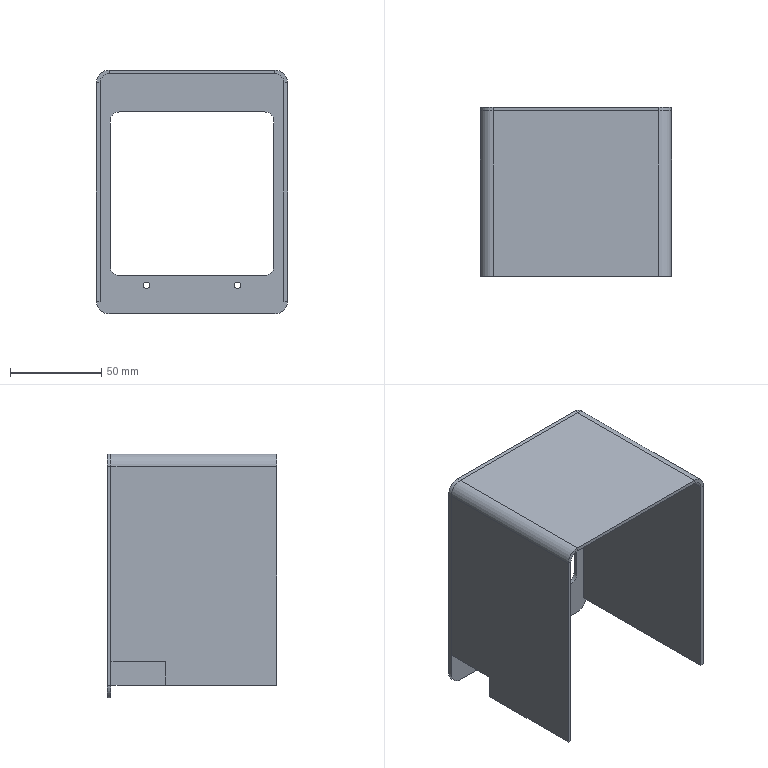Part | SolidWorks | features Cut 2, FlatPattern 2, SMBaseFlange 2, SheetMetal 2, HoleWzd 1 | 2 solids | 46 faces | box 105 x 93 x 134 mm | volume 74755 mm3 | plane 30 | cylinder 16 | commonest cylinder face diameters 10 x6 14 x6 3.4 x4
STEP:
#1=CARTESIAN_POINT('',(-45.5,91.,65.));
#2=VERTEX_POINT('',#1);
#3=CARTESIAN_POINT('',(-45.5,91.,67.));
#4=VERTEX_POINT('',#3);
#5=CARTESIAN_POINT('',(-45.5,91.,65.));
#6=DIRECTION('',(0.,0.,1.));
#7=VECTOR('',#6,1000.);
#8=LINE('',#5,#7);
#9=EDGE_CURVE('',#2,#4,#8,.T.);
#10=ORIENTED_EDGE('',*,*,#9,.F.);
#11=CARTESIAN_POINT('',(-50.5,91.,60.));
#12=VERTEX_POINT('',#11);
#13=CARTESIAN_POINT('',(-45.5,91.,60.));
#14=DIRECTION('',(0.,1.,0.));
#15=DIRECTION('',(0.,0.,1.));
#16=AXIS2_PLACEMENT_3D('',#13,#14,#15);
#17=CIRCLE('',#16,5.);
#18=EDGE_CURVE('',#12,#2,#17,.T.);
#19=ORIENTED_EDGE('',*,*,#18,.F.);
#20=CARTESIAN_POINT('',(-52.5,91.,60.));
#21=VERTEX_POINT('',#20);
#22=CARTESIAN_POINT('',(-52.5,91.,60.));
#23=DIRECTION('',(1.,0.,0.));
#24=VECTOR('',#23,1000.);
#25=LINE('',#22,#24);
#26=EDGE_CURVE('',#21,#12,#25,.T.);
#27=ORIENTED_EDGE('',*,*,#26,.F.);
#28=CARTESIAN_POINT('',(-45.5,91.,60.));
#29=DIRECTION('',(0.,1.,0.));
#30=DIRECTION('',(1.,0.,0.));
#31=AXIS2_PLACEMENT_3D('',#28,#29,#30);
#32=CIRCLE('',#31,7.);
#33=EDGE_CURVE('',#21,#4,#32,.T.);
#34=ORIENTED_EDGE('',*,*,#33,.T.);
#35=EDGE_LOOP('',(#10,#19,#27,#34));
#36=FACE_OUTER_BOUND('',#35,.T.);
#37=CARTESIAN_POINT('',(-45.5,91.,65.));
#38=DIRECTION('',(0.,1.,0.));
#39=DIRECTION('',(0.,0.,1.));
#40=AXIS2_PLACEMENT_3D('',#37,#38,#39);
#41=PLANE('',#40);
#42=ADVANCED_FACE('',(#36),#41,.T.);
#43=CARTESIAN_POINT('',(45.5,91.,65.));
#44=VERTEX_POINT('',#43);
#45=CARTESIAN_POINT('',(-45.5,91.,65.));
#46=DIRECTION('',(1.,0.,0.));
#47=VECTOR('',#46,1000.);
#48=LINE('',#45,#47);
#49=EDGE_CURVE('',#2,#44,#48,.T.);
#50=ORIENTED_EDGE('',*,*,#49,.F.);
#51=ORIENTED_EDGE('',*,*,#9,.T.);
#52=CARTESIAN_POINT('',(45.5,91.,67.));
#53=VERTEX_POINT('',#52);
#54=CARTESIAN_POINT('',(-45.5,91.,67.));
#55=DIRECTION('',(1.,0.,0.));
#56=VECTOR('',#55,1000.);
#57=LINE('',#54,#56);
#58=EDGE_CURVE('',#4,#53,#57,.T.);
#59=ORIENTED_EDGE('',*,*,#58,.T.);
#60=CARTESIAN_POINT('',(45.5,91.,67.));
#61=DIRECTION('',(0.,0.,-1.));
#62=VECTOR('',#61,1000.);
#63=LINE('',#60,#62);
#64=EDGE_CURVE('',#53,#44,#63,.T.);
#65=ORIENTED_EDGE('',*,*,#64,.T.);
#66=EDGE_LOOP('',(#50,#51,#59,#65));
#67=FACE_OUTER_BOUND('',#66,.T.);
#68=CARTESIAN_POINT('',(-52.5,91.,60.));
#69=DIRECTION('',(0.,1.,0.));
#70=DIRECTION('',(0.,0.,1.));
#71=AXIS2_PLACEMENT_3D('',#68,#69,#70);
#72=PLANE('',#71);
#73=ADVANCED_FACE('',(#67),#72,.T.);
#74=CARTESIAN_POINT('',(-50.5,0.,60.));
#75=VERTEX_POINT('',#74);
#76=CARTESIAN_POINT('',(-52.5,0.,60.));
#77=VERTEX_POINT('',#76);
#78=CARTESIAN_POINT('',(-50.5,0.,60.));
#79=DIRECTION('',(-1.,0.,0.));
#80=VECTOR('',#79,1000.);
#81=LINE('',#78,#80);
#82=EDGE_CURVE('',#75,#77,#81,.T.);
#83=ORIENTED_EDGE('',*,*,#82,.F.);
#84=CARTESIAN_POINT('',(-45.5,0.,65.));
#85=VERTEX_POINT('',#84);
#86=CARTESIAN_POINT('',(-45.5,0.,60.));
#87=DIRECTION('',(0.,1.,0.));
#88=DIRECTION('',(0.,0.,1.));
#89=AXIS2_PLACEMENT_3D('',#86,#87,#88);
#90=CIRCLE('',#89,5.);
#91=EDGE_CURVE('',#75,#85,#90,.T.);
#92=ORIENTED_EDGE('',*,*,#91,.T.);
#93=CARTESIAN_POINT('',(-45.5,0.,67.));
#94=VERTEX_POINT('',#93);
#95=CARTESIAN_POINT('',(-45.5,0.,67.));
#96=DIRECTION('',(0.,0.,-1.));
#97=VECTOR('',#96,1000.);
#98=LINE('',#95,#97);
#99=EDGE_CURVE('',#94,#85,#98,.T.);
#100=ORIENTED_EDGE('',*,*,#99,.F.);
#101=CARTESIAN_POINT('',(-45.5,0.,60.));
#102=DIRECTION('',(0.,1.,0.));
#103=DIRECTION('',(1.,0.,0.));
#104=AXIS2_PLACEMENT_3D('',#101,#102,#103);
#105=CIRCLE('',#104,7.);
#106=EDGE_CURVE('',#77,#94,#105,.T.);
#107=ORIENTED_EDGE('',*,*,#106,.F.);
#108=EDGE_LOOP('',(#83,#92,#100,#107));
#109=FACE_OUTER_BOUND('',#108,.T.);
#110=CARTESIAN_POINT('',(-50.5,0.,60.));
#111=DIRECTION('',(0.,-1.,0.));
#112=DIRECTION('',(0.,0.,-1.));
#113=AXIS2_PLACEMENT_3D('',#110,#111,#112);
#114=PLANE('',#113);
#115=ADVANCED_FACE('',(#109),#114,.T.);
#116=CARTESIAN_POINT('',(-50.5,0.,-60.));
#117=VERTEX_POINT('',#116);
#118=CARTESIAN_POINT('',(-50.5,0.,-60.));
#119=DIRECTION('',(0.,0.,1.));
#120=VECTOR('',#119,1000.);
#121=LINE('',#118,#120);
#122=EDGE_CURVE('',#117,#75,#121,.T.);
#123=ORIENTED_EDGE('',*,*,#122,.T.);
#124=ORIENTED_EDGE('',*,*,#82,.T.);
#125=CARTESIAN_POINT('',(-52.5,0.,-60.));
#126=VERTEX_POINT('',#125);
#127=CARTESIAN_POINT('',(-52.5,0.,-60.));
#128=DIRECTION('',(0.,0.,1.));
#129=VECTOR('',#128,1000.);
#130=LINE('',#127,#129);
#131=EDGE_CURVE('',#126,#77,#130,.T.);
#132=ORIENTED_EDGE('',*,*,#131,.F.);
#133=CARTESIAN_POINT('',(-52.5,0.,-60.));
#134=DIRECTION('',(1.,0.,0.));
#135=VECTOR('',#134,1000.);
#136=LINE('',#133,#135);
#137=EDGE_CURVE('',#126,#117,#136,.T.);
#138=ORIENTED_EDGE('',*,*,#137,.T.);
#139=EDGE_LOOP('',(#123,#124,#132,#138));
#140=FACE_OUTER_BOUND('',#139,.T.);
#141=CARTESIAN_POINT('',(-45.5,0.,67.));
#142=DIRECTION('',(0.,-1.,0.));
#143=DIRECTION('',(0.,0.,-1.));
#144=AXIS2_PLACEMENT_3D('',#141,#142,#143);
#145=PLANE('',#144);
#146=ADVANCED_FACE('',(#140),#145,.T.);
#147=CARTESIAN_POINT('',(50.5,91.,60.));
#148=VERTEX_POINT('',#147);
#149=CARTESIAN_POINT('',(52.5,91.,60.));
#150=VERTEX_POINT('',#149);
#151=CARTESIAN_POINT('',(50.5,91.,60.));
#152=DIRECTION('',(1.,0.,0.));
#153=VECTOR('',#152,1000.);
#154=LINE('',#151,#153);
#155=EDGE_CURVE('',#148,#150,#154,.T.);
#156=ORIENTED_EDGE('',*,*,#155,.F.);
#157=CARTESIAN_POINT('',(45.5,91.,60.));
#158=DIRECTION('',(0.,1.,0.));
#159=DIRECTION('',(0.,0.,1.));
#160=AXIS2_PLACEMENT_3D('',#157,#158,#159);
#161=CIRCLE('',#160,5.);
#162=EDGE_CURVE('',#44,#148,#161,.T.);
#163=ORIENTED_EDGE('',*,*,#162,.F.);
#164=ORIENTED_EDGE('',*,*,#64,.F.);
#165=CARTESIAN_POINT('',(45.5,91.,60.));
#166=DIRECTION('',(0.,1.,0.));
#167=DIRECTION('',(1.,0.,0.));
#168=AXIS2_PLACEMENT_3D('',#165,#166,#167);
#169=CIRCLE('',#168,7.);
#170=EDGE_CURVE('',#53,#150,#169,.T.);
#171=ORIENTED_EDGE('',*,*,#170,.T.);
#172=EDGE_LOOP('',(#156,#163,#164,#171));
#173=FACE_OUTER_BOUND('',#172,.T.);
#174=CARTESIAN_POINT('',(50.5,91.,60.));
#175=DIRECTION('',(0.,1.,0.));
#176=DIRECTION('',(0.,0.,1.));
#177=AXIS2_PLACEMENT_3D('',#174,#175,#176);
#178=PLANE('',#177);
#179=ADVANCED_FACE('',(#173),#178,.T.);
#180=CARTESIAN_POINT('',(50.5,91.,-60.));
#181=VERTEX_POINT('',#180);
#182=CARTESIAN_POINT('',(50.5,91.,60.));
#183=DIRECTION('',(0.,0.,-1.));
#184=VECTOR('',#183,1000.);
#185=LINE('',#182,#184);
#186=EDGE_CURVE('',#148,#181,#185,.T.);
#187=ORIENTED_EDGE('',*,*,#186,.F.);
#188=ORIENTED_EDGE('',*,*,#155,.T.);
#189=CARTESIAN_POINT('',(52.5,91.,-60.));
#190=VERTEX_POINT('',#189);
#191=CARTESIAN_POINT('',(52.5,91.,60.));
#192=DIRECTION('',(0.,0.,-1.));
#193=VECTOR('',#192,1000.);
#194=LINE('',#191,#193);
#195=EDGE_CURVE('',#150,#190,#194,.T.);
#196=ORIENTED_EDGE('',*,*,#195,.T.);
#197=CARTESIAN_POINT('',(50.5,91.,-60.));
#198=DIRECTION('',(1.,0.,0.));
#199=VECTOR('',#198,1000.);
#200=LINE('',#197,#199);
#201=EDGE_CURVE('',#181,#190,#200,.T.);
#202=ORIENTED_EDGE('',*,*,#201,.F.);
#203=EDGE_LOOP('',(#187,#188,#196,#202));
#204=FACE_OUTER_BOUND('',#203,.T.);
#205=CARTESIAN_POINT('',(45.5,91.,67.));
#206=DIRECTION('',(0.,1.,0.));
#207=DIRECTION('',(0.,0.,1.));
#208=AXIS2_PLACEMENT_3D('',#205,#206,#207);
#209=PLANE('',#208);
#210=ADVANCED_FACE('',(#204),#209,.T.);
#211=CARTESIAN_POINT('',(45.5,0.,65.));
#212=VERTEX_POINT('',#211);
#213=CARTESIAN_POINT('',(45.5,0.,67.));
#214=VERTEX_POINT('',#213);
#215=CARTESIAN_POINT('',(45.5,0.,65.));
#216=DIRECTION('',(0.,0.,1.));
#217=VECTOR('',#216,1000.);
#218=LINE('',#215,#217);
#219=EDGE_CURVE('',#212,#214,#218,.T.);
#220=ORIENTED_EDGE('',*,*,#219,.F.);
#221=CARTESIAN_POINT('',(50.5,0.,60.));
#222=VERTEX_POINT('',#221);
#223=CARTESIAN_POINT('',(45.5,0.,60.));
#224=DIRECTION('',(0.,1.,0.));
#225=DIRECTION('',(0.,0.,1.));
#226=AXIS2_PLACEMENT_3D('',#223,#224,#225);
#227=CIRCLE('',#226,5.);
#228=EDGE_CURVE('',#212,#222,#227,.T.);
#229=ORIENTED_EDGE('',*,*,#228,.T.);
#230=CARTESIAN_POINT('',(52.5,0.,60.));
#231=VERTEX_POINT('',#230);
#232=CARTESIAN_POINT('',(52.5,0.,60.));
#233=DIRECTION('',(-1.,0.,0.));
#234=VECTOR('',#233,1000.);
#235=LINE('',#232,#234);
#236=EDGE_CURVE('',#231,#222,#235,.T.);
#237=ORIENTED_EDGE('',*,*,#236,.F.);
#238=CARTESIAN_POINT('',(45.5,0.,60.));
#239=DIRECTION('',(0.,1.,0.));
#240=DIRECTION('',(1.,0.,0.));
#241=AXIS2_PLACEMENT_3D('',#238,#239,#240);
#242=CIRCLE('',#241,7.);
#243=EDGE_CURVE('',#214,#231,#242,.T.);
#244=ORIENTED_EDGE('',*,*,#243,.F.);
#245=EDGE_LOOP('',(#220,#229,#237,#244));
#246=FACE_OUTER_BOUND('',#245,.T.);
#247=CARTESIAN_POINT('',(45.5,0.,65.));
#248=DIRECTION('',(0.,-1.,0.));
#249=DIRECTION('',(0.,0.,-1.));
#250=AXIS2_PLACEMENT_3D('',#247,#248,#249);
#251=PLANE('',#250);
#252=ADVANCED_FACE('',(#246),#251,.T.);
#253=CARTESIAN_POINT('',(-45.5,0.,65.));
#254=DIRECTION('',(1.,0.,0.));
#255=VECTOR('',#254,1000.);
#256=LINE('',#253,#255);
#257=EDGE_CURVE('',#85,#212,#256,.T.);
#258=ORIENTED_EDGE('',*,*,#257,.T.);
#259=ORIENTED_EDGE('',*,*,#219,.T.);
#260=CARTESIAN_POINT('',(-45.5,0.,67.));
#261=DIRECTION('',(1.,0.,0.));
#262=VECTOR('',#261,1000.);
#263=LINE('',#260,#262);
#264=EDGE_CURVE('',#94,#214,#263,.T.);
#265=ORIENTED_EDGE('',*,*,#264,.F.);
#266=ORIENTED_EDGE('',*,*,#99,.T.);
#267=EDGE_LOOP('',(#258,#259,#265,#266));
#268=FACE_OUTER_BOUND('',#267,.T.);
#269=CARTESIAN_POINT('',(52.5,0.,60.));
#270=DIRECTION('',(0.,-1.,0.));
#271=DIRECTION('',(0.,0.,-1.));
#272=AXIS2_PLACEMENT_3D('',#269,#270,#271);
#273=PLANE('',#272);
#274=ADVANCED_FACE('',(#268),#273,.T.);
#275=CARTESIAN_POINT('',(52.5,0.,-60.));
#276=VERTEX_POINT('',#275);
#277=CARTESIAN_POINT('',(52.5,0.,60.));
#278=DIRECTION('',(0.,0.,-1.));
#279=VECTOR('',#278,1000.);
#280=LINE('',#277,#279);
#281=EDGE_CURVE('',#231,#276,#280,.T.);
#282=ORIENTED_EDGE('',*,*,#281,.T.);
#283=CARTESIAN_POINT('',(52.5,91.,-60.));
#284=DIRECTION('',(0.,-1.,0.));
#285=VECTOR('',#284,1000.);
#286=LINE('',#283,#285);
#287=EDGE_CURVE('',#190,#276,#286,.T.);
#288=ORIENTED_EDGE('',*,*,#287,.F.);
#289=ORIENTED_EDGE('',*,*,#195,.F.);
#290=CARTESIAN_POINT('',(52.5,91.,60.));
#291=DIRECTION('',(0.,-1.,0.));
#292=VECTOR('',#291,1000.);
#293=LINE('',#290,#292);
#294=EDGE_CURVE('',#150,#231,#293,.T.);
#295=ORIENTED_EDGE('',*,*,#294,.T.);
#296=EDGE_LOOP('',(#282,#288,#289,#295));
#297=FACE_OUTER_BOUND('',#296,.T.);
#298=CARTESIAN_POINT('',(52.5,91.,60.));
#299=DIRECTION('',(-1.,0.,0.));
#300=DIRECTION('',(0.,0.,1.));
#301=AXIS2_PLACEMENT_3D('',#298,#299,#300);
#302=PLANE('',#301);
#303=ADVANCED_FACE('',(#297),#302,.F.);
#304=CARTESIAN_POINT('',(50.5,0.,-60.));
#305=VERTEX_POINT('',#304);
#306=CARTESIAN_POINT('',(50.5,0.,-60.));
#307=DIRECTION('',(1.,0.,0.));
#308=VECTOR('',#307,1000.);
#309=LINE('',#306,#308);
#310=EDGE_CURVE('',#305,#276,#309,.T.);
#311=ORIENTED_EDGE('',*,*,#310,.F.);
#312=CARTESIAN_POINT('',(50.5,91.,-60.));
#313=DIRECTION('',(0.,-1.,0.));
#314=VECTOR('',#313,1000.);
#315=LINE('',#312,#314);
#316=EDGE_CURVE('',#181,#305,#315,.T.);
#317=ORIENTED_EDGE('',*,*,#316,.F.);
#318=ORIENTED_EDGE('',*,*,#201,.T.);
#319=ORIENTED_EDGE('',*,*,#287,.T.);
#320=EDGE_LOOP('',(#311,#317,#318,#319));
#321=FACE_OUTER_BOUND('',#320,.T.);
#322=CARTESIAN_POINT('',(50.5,91.,-60.));
#323=DIRECTION('',(0.,0.,-1.));
#324=DIRECTION('',(-1.,0.,0.));
#325=AXIS2_PLACEMENT_3D('',#322,#323,#324);
#326=PLANE('',#325);
#327=ADVANCED_FACE('',(#321),#326,.T.);
#328=CARTESIAN_POINT('',(50.5,0.,60.));
#329=DIRECTION('',(0.,0.,-1.));
#330=VECTOR('',#329,1000.);
#331=LINE('',#328,#330);
#332=EDGE_CURVE('',#222,#305,#331,.T.);
#333=ORIENTED_EDGE('',*,*,#332,.F.);
#334=CARTESIAN_POINT('',(50.5,91.,60.));
#335=DIRECTION('',(0.,-1.,0.));
#336=VECTOR('',#335,1000.);
#337=LINE('',#334,#336);
#338=EDGE_CURVE('',#148,#222,#337,.T.);
#339=ORIENTED_EDGE('',*,*,#338,.F.);
#340=ORIENTED_EDGE('',*,*,#186,.T.);
#341=ORIENTED_EDGE('',*,*,#316,.T.);
#342=EDGE_LOOP('',(#333,#339,#340,#341));
#343=FACE_OUTER_BOUND('',#342,.T.);
#344=CARTESIAN_POINT('',(50.5,91.,60.));
#345=DIRECTION('',(-1.,0.,0.));
#346=DIRECTION('',(0.,0.,1.));
#347=AXIS2_PLACEMENT_3D('',#344,#345,#346);
#348=PLANE('',#347);
#349=ADVANCED_FACE('',(#343),#348,.T.);
#350=ORIENTED_EDGE('',*,*,#228,.F.);
#351=CARTESIAN_POINT('',(45.5,91.,65.));
#352=DIRECTION('',(0.,-1.,0.));
#353=VECTOR('',#352,1000.);
#354=LINE('',#351,#353);
#355=EDGE_CURVE('',#44,#212,#354,.T.);
#356=ORIENTED_EDGE('',*,*,#355,.F.);
#357=ORIENTED_EDGE('',*,*,#162,.T.);
#358=ORIENTED_EDGE('',*,*,#338,.T.);
#359=EDGE_LOOP('',(#350,#356,#357,#358));
#360=FACE_OUTER_BOUND('',#359,.T.);
#361=CARTESIAN_POINT('',(45.5,91.,60.));
#362=DIRECTION('',(0.,-1.,0.));
#363=DIRECTION('',(0.,0.,-1.));
#364=AXIS2_PLACEMENT_3D('',#361,#362,#363);
#365=CYLINDRICAL_SURFACE('',#364,5.);
#366=ADVANCED_FACE('',(#360),#365,.F.);
#367=ORIENTED_EDGE('',*,*,#257,.F.);
#368=CARTESIAN_POINT('',(-45.5,91.,65.));
#369=DIRECTION('',(0.,-1.,0.));
#370=VECTOR('',#369,1000.);
#371=LINE('',#368,#370);
#372=EDGE_CURVE('',#2,#85,#371,.T.);
#373=ORIENTED_EDGE('',*,*,#372,.F.);
#374=ORIENTED_EDGE('',*,*,#49,.T.);
#375=ORIENTED_EDGE('',*,*,#355,.T.);
#376=EDGE_LOOP('',(#367,#373,#374,#375));
#377=FACE_OUTER_BOUND('',#376,.T.);
#378=CARTESIAN_POINT('',(-45.5,91.,65.));
#379=DIRECTION('',(0.,0.,-1.));
#380=DIRECTION('',(-1.,0.,0.));
#381=AXIS2_PLACEMENT_3D('',#378,#379,#380);
#382=PLANE('',#381);
#383=ADVANCED_FACE('',(#377),#382,.T.);
#384=ORIENTED_EDGE('',*,*,#91,.F.);
#385=CARTESIAN_POINT('',(-50.5,91.,60.));
#386=DIRECTION('',(0.,-1.,0.));
#387=VECTOR('',#386,1000.);
#388=LINE('',#385,#387);
#389=EDGE_CURVE('',#12,#75,#388,.T.);
#390=ORIENTED_EDGE('',*,*,#389,.F.);
#391=ORIENTED_EDGE('',*,*,#18,.T.);
#392=ORIENTED_EDGE('',*,*,#372,.T.);
#393=EDGE_LOOP('',(#384,#390,#391,#392));
#394=FACE_OUTER_BOUND('',#393,.T.);
#395=CARTESIAN_POINT('',(-45.5,91.,60.));
#396=DIRECTION('',(0.,-1.,0.));
#397=DIRECTION('',(0.,0.,-1.));
#398=AXIS2_PLACEMENT_3D('',#395,#396,#397);
#399=CYLINDRICAL_SURFACE('',#398,5.);
#400=ADVANCED_FACE('',(#394),#399,.F.);
#401=CARTESIAN_POINT('',(-50.5,61.,-60.));
#402=VERTEX_POINT('',#401);
#403=CARTESIAN_POINT('',(-50.5,61.,-47.));
#404=VERTEX_POINT('',#403);
#405=CARTESIAN_POINT('',(-50.5,61.,-60.));
#406=DIRECTION('',(0.,0.,1.));
#407=VECTOR('',#406,1000.);
#408=LINE('',#405,#407);
#409=EDGE_CURVE('',#402,#404,#408,.T.);
#410=ORIENTED_EDGE('',*,*,#409,.T.);
#411=CARTESIAN_POINT('',(-50.5,91.,-47.));
#412=VERTEX_POINT('',#411);
#413=CARTESIAN_POINT('',(-50.5,91.,-47.));
#414=DIRECTION('',(0.,1.,0.));
#415=VECTOR('',#414,1000.);
#416=LINE('',#413,#415);
#417=EDGE_CURVE('',#404,#412,#416,.T.);
#418=ORIENTED_EDGE('',*,*,#417,.T.);
#419=CARTESIAN_POINT('',(-50.5,91.,-60.));
#420=DIRECTION('',(0.,0.,1.));
#421=VECTOR('',#420,1000.);
#422=LINE('',#419,#421);
#423=EDGE_CURVE('',#412,#12,#422,.T.);
#424=ORIENTED_EDGE('',*,*,#423,.T.);
#425=ORIENTED_EDGE('',*,*,#389,.T.);
#426=ORIENTED_EDGE('',*,*,#122,.F.);
#427=CARTESIAN_POINT('',(-50.5,91.,-60.));
#428=DIRECTION('',(0.,-1.,0.));
#429=VECTOR('',#428,1000.);
#430=LINE('',#427,#429);
#431=EDGE_CURVE('',#402,#117,#430,.T.);
#432=ORIENTED_EDGE('',*,*,#431,.F.);
#433=EDGE_LOOP('',(#410,#418,#424,#425,#426,#432));
#434=FACE_OUTER_BOUND('',#433,.T.);
#435=CARTESIAN_POINT('',(-50.5,91.,-60.));
#436=DIRECTION('',(1.,0.,0.));
#437=DIRECTION('',(0.,0.,-1.));
#438=AXIS2_PLACEMENT_3D('',#435,#436,#437);
#439=PLANE('',#438);
#440=ADVANCED_FACE('',(#434),#439,.T.);
#441=CARTESIAN_POINT('',(-52.5,61.,-60.));
#442=VERTEX_POINT('',#441);
#443=CARTESIAN_POINT('',(52.501,61.,-60.));
#444=DIRECTION('',(-1.,0.,0.));
#445=VECTOR('',#444,1000.);
#446=LINE('',#443,#445);
#447=EDGE_CURVE('',#402,#442,#446,.T.);
#448=ORIENTED_EDGE('',*,*,#447,.F.);
#449=ORIENTED_EDGE('',*,*,#431,.T.);
#450=ORIENTED_EDGE('',*,*,#137,.F.);
#451=CARTESIAN_POINT('',(-52.5,91.,-60.));
#452=DIRECTION('',(0.,-1.,0.));
#453=VECTOR('',#452,1000.);
#454=LINE('',#451,#453);
#455=EDGE_CURVE('',#442,#126,#454,.T.);
#456=ORIENTED_EDGE('',*,*,#455,.F.);
#457=EDGE_LOOP('',(#448,#449,#450,#456));
#458=FACE_OUTER_BOUND('',#457,.T.);
#459=CARTESIAN_POINT('',(-52.5,91.,-60.));
#460=DIRECTION('',(0.,0.,-1.));
#461=DIRECTION('',(-1.,0.,0.));
#462=AXIS2_PLACEMENT_3D('',#459,#460,#461);
#463=PLANE('',#462);
#464=ADVANCED_FACE('',(#458),#463,.T.);
#465=CARTESIAN_POINT('',(-52.5,61.,-47.));
#466=VERTEX_POINT('',#465);
#467=CARTESIAN_POINT('',(-52.5,91.,-47.));
#468=VERTEX_POINT('',#467);
#469=CARTESIAN_POINT('',(-52.5,91.,-47.));
#470=DIRECTION('',(0.,1.,0.));
#471=VECTOR('',#470,1000.);
#472=LINE('',#469,#471);
#473=EDGE_CURVE('',#466,#468,#472,.T.);
#474=ORIENTED_EDGE('',*,*,#473,.F.);
#475=CARTESIAN_POINT('',(-52.5,61.,-60.));
#476=DIRECTION('',(0.,0.,1.));
#477=VECTOR('',#476,1000.);
#478=LINE('',#475,#477);
#479=EDGE_CURVE('',#442,#466,#478,.T.);
#480=ORIENTED_EDGE('',*,*,#479,.F.);
#481=ORIENTED_EDGE('',*,*,#455,.T.);
#482=ORIENTED_EDGE('',*,*,#131,.T.);
#483=CARTESIAN_POINT('',(-52.5,91.,60.));
#484=DIRECTION('',(0.,-1.,0.));
#485=VECTOR('',#484,1000.);
#486=LINE('',#483,#485);
#487=EDGE_CURVE('',#21,#77,#486,.T.);
#488=ORIENTED_EDGE('',*,*,#487,.F.);
#489=CARTESIAN_POINT('',(-52.5,91.,-60.));
#490=DIRECTION('',(0.,0.,1.));
#491=VECTOR('',#490,1000.);
#492=LINE('',#489,#491);
#493=EDGE_CURVE('',#468,#21,#492,.T.);
#494=ORIENTED_EDGE('',*,*,#493,.F.);
#495=EDGE_LOOP('',(#474,#480,#481,#482,#488,#494));
#496=FACE_OUTER_BOUND('',#495,.T.);
#497=CARTESIAN_POINT('',(-52.5,91.,-60.));
#498=DIRECTION('',(1.,0.,0.));
#499=DIRECTION('',(0.,0.,-1.));
#500=AXIS2_PLACEMENT_3D('',#497,#498,#499);
#501=PLANE('',#500);
#502=ADVANCED_FACE('',(#496),#501,.F.);
#503=ORIENTED_EDGE('',*,*,#106,.T.);
#504=CARTESIAN_POINT('',(-45.5,91.,67.));
#505=DIRECTION('',(0.,-1.,0.));
#506=VECTOR('',#505,1000.);
#507=LINE('',#504,#506);
#508=EDGE_CURVE('',#4,#94,#507,.T.);
#509=ORIENTED_EDGE('',*,*,#508,.F.);
#510=ORIENTED_EDGE('',*,*,#33,.F.);
#511=ORIENTED_EDGE('',*,*,#487,.T.);
#512=EDGE_LOOP('',(#503,#509,#510,#511));
#513=FACE_OUTER_BOUND('',#512,.T.);
#514=CARTESIAN_POINT('',(-45.5,91.,60.));
#515=DIRECTION('',(0.,-1.,0.));
#516=DIRECTION('',(0.,0.,-1.));
#517=AXIS2_PLACEMENT_3D('',#514,#515,#516);
#518=CYLINDRICAL_SURFACE('',#517,7.);
#519=ADVANCED_FACE('',(#513),#518,.T.);
#520=ORIENTED_EDGE('',*,*,#264,.T.);
#521=CARTESIAN_POINT('',(45.5,91.,67.));
#522=DIRECTION('',(0.,-1.,0.));
#523=VECTOR('',#522,1000.);
#524=LINE('',#521,#523);
#525=EDGE_CURVE('',#53,#214,#524,.T.);
#526=ORIENTED_EDGE('',*,*,#525,.F.);
#527=ORIENTED_EDGE('',*,*,#58,.F.);
#528=ORIENTED_EDGE('',*,*,#508,.T.);
#529=EDGE_LOOP('',(#520,#526,#527,#528));
#530=FACE_OUTER_BOUND('',#529,.T.);
#531=CARTESIAN_POINT('',(-45.5,91.,67.));
#532=DIRECTION('',(0.,0.,-1.));
#533=DIRECTION('',(-1.,0.,0.));
#534=AXIS2_PLACEMENT_3D('',#531,#532,#533);
#535=PLANE('',#534);
#536=ADVANCED_FACE('',(#530),#535,.F.);
#537=ORIENTED_EDGE('',*,*,#243,.T.);
#538=ORIENTED_EDGE('',*,*,#294,.F.);
#539=ORIENTED_EDGE('',*,*,#170,.F.);
#540=ORIENTED_EDGE('',*,*,#525,.T.);
#541=EDGE_LOOP('',(#537,#538,#539,#540));
#542=FACE_OUTER_BOUND('',#541,.T.);
#543=CARTESIAN_POINT('',(45.5,91.,60.));
#544=DIRECTION('',(0.,-1.,0.));
#545=DIRECTION('',(0.,0.,-1.));
#546=AXIS2_PLACEMENT_3D('',#543,#544,#545);
#547=CYLINDRICAL_SURFACE('',#546,7.);
#548=ADVANCED_FACE('',(#542),#547,.T.);
#549=CARTESIAN_POINT('',(52.501,91.,-47.));
#550=DIRECTION('',(-1.,0.,0.));
#551=VECTOR('',#550,1000.);
#552=LINE('',#549,#551);
#553=EDGE_CURVE('',#412,#468,#552,.T.);
#554=ORIENTED_EDGE('',*,*,#553,.T.);
#555=ORIENTED_EDGE('',*,*,#493,.T.);
#556=ORIENTED_EDGE('',*,*,#26,.T.);
#557=ORIENTED_EDGE('',*,*,#423,.F.);
#558=EDGE_LOOP('',(#554,#555,#556,#557));
#559=FACE_OUTER_BOUND('',#558,.T.);
#560=CARTESIAN_POINT('',(45.5,91.,60.));
#561=DIRECTION('',(0.,1.,0.));
#562=DIRECTION('',(1.,0.,0.));
#563=AXIS2_PLACEMENT_3D('',#560,#561,#562);
#564=PLANE('',#563);
#565=ADVANCED_FACE('',(#559),#564,.T.);
#566=ORIENTED_EDGE('',*,*,#281,.F.);
#567=ORIENTED_EDGE('',*,*,#236,.T.);
#568=ORIENTED_EDGE('',*,*,#332,.T.);
#569=ORIENTED_EDGE('',*,*,#310,.T.);
#570=EDGE_LOOP('',(#566,#567,#568,#569));
#571=FACE_OUTER_BOUND('',#570,.T.);
#572=CARTESIAN_POINT('',(45.5,0.,60.));
#573=DIRECTION('',(0.,1.,0.));
#574=DIRECTION('',(1.,0.,0.));
#575=AXIS2_PLACEMENT_3D('',#572,#573,#574);
#576=PLANE('',#575);
#577=ADVANCED_FACE('',(#571),#576,.F.);
#578=ORIENTED_EDGE('',*,*,#447,.T.);
#579=ORIENTED_EDGE('',*,*,#479,.T.);
#580=CARTESIAN_POINT('',(52.501,61.,-47.));
#581=DIRECTION('',(-1.,0.,0.));
#582=VECTOR('',#581,1000.);
#583=LINE('',#580,#582);
#584=EDGE_CURVE('',#404,#466,#583,.T.);
#585=ORIENTED_EDGE('',*,*,#584,.F.);
#586=ORIENTED_EDGE('',*,*,#409,.F.);
#587=EDGE_LOOP('',(#578,#579,#585,#586));
#588=FACE_OUTER_BOUND('',#587,.T.);
#589=CARTESIAN_POINT('',(52.501,61.,-60.));
#590=DIRECTION('',(0.,-1.,0.));
#591=DIRECTION('',(0.,0.,-1.));
#592=AXIS2_PLACEMENT_3D('',#589,#590,#591);
#593=PLANE('',#592);
#594=ADVANCED_FACE('',(#588),#593,.F.);
#595=ORIENTED_EDGE('',*,*,#584,.T.);
#596=ORIENTED_EDGE('',*,*,#473,.T.);
#597=ORIENTED_EDGE('',*,*,#553,.F.);
#598=ORIENTED_EDGE('',*,*,#417,.F.);
#599=EDGE_LOOP('',(#595,#596,#597,#598));
#600=FACE_OUTER_BOUND('',#599,.T.);
#601=CARTESIAN_POINT('',(52.501,91.,-47.));
#602=DIRECTION('',(0.,0.,1.));
#603=DIRECTION('',(0.,-1.,0.));
#604=AXIS2_PLACEMENT_3D('',#601,#602,#603);
#605=PLANE('',#604);
#606=ADVANCED_FACE('',(#600),#605,.F.);
#607=CLOSED_SHELL('',(#42,#73,#115,#146,#179,#210,#252,#274,#303,#327,#349,#366,#383,#400,#440,#464,#502,#519,#536,#548,#565,#577,#594,#606));
#608=MANIFOLD_SOLID_BREP('',#607);
#609=CARTESIAN_POINT('',(-25.,91.,-52.93));
#610=VERTEX_POINT('',#609);
#611=CARTESIAN_POINT('',(-25.,91.,-49.53));
#612=VERTEX_POINT('',#611);
#613=CARTESIAN_POINT('',(-25.,91.,-51.23));
#614=DIRECTION('',(0.,1.,0.));
#615=DIRECTION('',(0.,0.,1.));
#616=AXIS2_PLACEMENT_3D('',#613,#614,#615);
#617=CIRCLE('',#616,1.7);
#618=EDGE_CURVE('',#610,#612,#617,.T.);
#619=ORIENTED_EDGE('',*,*,#618,.F.);
#620=CARTESIAN_POINT('',(-25.,93.,-52.93));
#621=VERTEX_POINT('',#620);
#622=CARTESIAN_POINT('',(-25.,93.,-52.93));
#623=DIRECTION('',(0.,1.,0.));
#624=VECTOR('',#623,1000.);
#625=LINE('',#622,#624);
#626=EDGE_CURVE('',#610,#621,#625,.T.);
#627=ORIENTED_EDGE('',*,*,#626,.T.);
#628=CARTESIAN_POINT('',(-25.,93.,-49.53));
#629=VERTEX_POINT('',#628);
#630=CARTESIAN_POINT('',(-25.,93.,-51.23));
#631=DIRECTION('',(0.,1.,0.));
#632=DIRECTION('',(0.,0.,1.));
#633=AXIS2_PLACEMENT_3D('',#630,#631,#632);
#634=CIRCLE('',#633,1.7);
#635=EDGE_CURVE('',#621,#629,#634,.T.);
#636=ORIENTED_EDGE('',*,*,#635,.T.);
#637=CARTESIAN_POINT('',(-25.,93.,-49.53));
#638=DIRECTION('',(0.,1.,0.));
#639=VECTOR('',#638,1000.);
#640=LINE('',#637,#639);
#641=EDGE_CURVE('',#612,#629,#640,.T.);
#642=ORIENTED_EDGE('',*,*,#641,.F.);
#643=EDGE_LOOP('',(#619,#627,#636,#642));
#644=FACE_OUTER_BOUND('',#643,.T.);
#645=CARTESIAN_POINT('',(-25.,93.,-51.23));
#646=DIRECTION('',(0.,1.,0.));
#647=DIRECTION('',(0.,0.,1.));
#648=AXIS2_PLACEMENT_3D('',#645,#646,#647);
#649=CYLINDRICAL_SURFACE('',#648,1.7);
#650=ADVANCED_FACE('',(#644),#649,.F.);
#651=CARTESIAN_POINT('',(25.,91.,-52.93));
#652=VERTEX_POINT('',#651);
#653=CARTESIAN_POINT('',(25.,91.,-49.53));
#654=VERTEX_POINT('',#653);
#655=CARTESIAN_POINT('',(25.,91.,-51.23));
#656=DIRECTION('',(0.,1.,0.));
#657=DIRECTION('',(0.,0.,1.));
#658=AXIS2_PLACEMENT_3D('',#655,#656,#657);
#659=CIRCLE('',#658,1.7);
#660=EDGE_CURVE('',#652,#654,#659,.T.);
#661=ORIENTED_EDGE('',*,*,#660,.F.);
#662=CARTESIAN_POINT('',(25.,93.,-52.93));
#663=VERTEX_POINT('',#662);
#664=CARTESIAN_POINT('',(25.,93.,-52.93));
#665=DIRECTION('',(0.,1.,0.));
#666=VECTOR('',#665,1000.);
#667=LINE('',#664,#666);
#668=EDGE_CURVE('',#652,#663,#667,.T.);
#669=ORIENTED_EDGE('',*,*,#668,.T.);
#670=CARTESIAN_POINT('',(25.,93.,-49.53));
#671=VERTEX_POINT('',#670);
#672=CARTESIAN_POINT('',(25.,93.,-51.23));
#673=DIRECTION('',(0.,1.,0.));
#674=DIRECTION('',(0.,0.,1.));
#675=AXIS2_PLACEMENT_3D('',#672,#673,#674);
#676=CIRCLE('',#675,1.7);
#677=EDGE_CURVE('',#663,#671,#676,.T.);
#678=ORIENTED_EDGE('',*,*,#677,.T.);
#679=CARTESIAN_POINT('',(25.,93.,-49.53));
#680=DIRECTION('',(0.,1.,0.));
#681=VECTOR('',#680,1000.);
#682=LINE('',#679,#681);
#683=EDGE_CURVE('',#654,#671,#682,.T.);
#684=ORIENTED_EDGE('',*,*,#683,.F.);
#685=EDGE_LOOP('',(#661,#669,#678,#684));
#686=FACE_OUTER_BOUND('',#685,.T.);
#687=CARTESIAN_POINT('',(25.,93.,-51.23));
#688=DIRECTION('',(0.,1.,0.));
#689=DIRECTION('',(0.,0.,1.));
#690=AXIS2_PLACEMENT_3D('',#687,#688,#689);
#691=CYLINDRICAL_SURFACE('',#690,1.7);
#692=ADVANCED_FACE('',(#686),#691,.F.);
#693=CARTESIAN_POINT('',(52.5,91.,-60.));
#694=VERTEX_POINT('',#693);
#695=CARTESIAN_POINT('',(45.5,91.,-67.));
#696=VERTEX_POINT('',#695);
#697=CARTESIAN_POINT('',(45.5,91.,-60.));
#698=DIRECTION('',(0.,1.,0.));
#699=DIRECTION('',(0.,0.,1.));
#700=AXIS2_PLACEMENT_3D('',#697,#698,#699);
#701=CIRCLE('',#700,7.);
#702=EDGE_CURVE('',#694,#696,#701,.T.);
#703=ORIENTED_EDGE('',*,*,#702,.T.);
#704=CARTESIAN_POINT('',(45.5,93.,-67.));
#705=VERTEX_POINT('',#704);
#706=CARTESIAN_POINT('',(45.5,93.,-67.));
#707=DIRECTION('',(0.,-1.,0.));
#708=VECTOR('',#707,1000.);
#709=LINE('',#706,#708);
#710=EDGE_CURVE('',#705,#696,#709,.T.);
#711=ORIENTED_EDGE('',*,*,#710,.F.);
#712=CARTESIAN_POINT('',(52.5,93.,-60.));
#713=VERTEX_POINT('',#712);
#714=CARTESIAN_POINT('',(45.5,93.,-60.));
#715=DIRECTION('',(0.,1.,0.));
#716=DIRECTION('',(0.,0.,1.));
#717=AXIS2_PLACEMENT_3D('',#714,#715,#716);
#718=CIRCLE('',#717,7.);
#719=EDGE_CURVE('',#713,#705,#718,.T.);
#720=ORIENTED_EDGE('',*,*,#719,.F.);
#721=CARTESIAN_POINT('',(52.5,93.,-60.));
#722=DIRECTION('',(0.,-1.,0.));
#723=VECTOR('',#722,1000.);
#724=LINE('',#721,#723);
#725=EDGE_CURVE('',#713,#694,#724,.T.);
#726=ORIENTED_EDGE('',*,*,#725,.T.);
#727=EDGE_LOOP('',(#703,#711,#720,#726));
#728=FACE_OUTER_BOUND('',#727,.T.);
#729=CARTESIAN_POINT('',(45.5,93.,-60.));
#730=DIRECTION('',(0.,-1.,0.));
#731=DIRECTION('',(0.,0.,-1.));
#732=AXIS2_PLACEMENT_3D('',#729,#730,#731);
#733=CYLINDRICAL_SURFACE('',#732,7.);
#734=ADVANCED_FACE('',(#728),#733,.T.);
#735=CARTESIAN_POINT('',(-45.5,91.,-67.));
#736=VERTEX_POINT('',#735);
#737=CARTESIAN_POINT('',(45.5,91.,-67.));
#738=DIRECTION('',(-1.,0.,0.));
#739=VECTOR('',#738,1000.);
#740=LINE('',#737,#739);
#741=EDGE_CURVE('',#696,#736,#740,.T.);
#742=ORIENTED_EDGE('',*,*,#741,.T.);
#743=CARTESIAN_POINT('',(-45.5,93.,-67.));
#744=VERTEX_POINT('',#743);
#745=CARTESIAN_POINT('',(-45.5,93.,-67.));
#746=DIRECTION('',(0.,-1.,0.));
#747=VECTOR('',#746,1000.);
#748=LINE('',#745,#747);
#749=EDGE_CURVE('',#744,#736,#748,.T.);
#750=ORIENTED_EDGE('',*,*,#749,.F.);
#751=CARTESIAN_POINT('',(45.5,93.,-67.));
#752=DIRECTION('',(-1.,0.,0.));
#753=VECTOR('',#752,1000.);
#754=LINE('',#751,#753);
#755=EDGE_CURVE('',#705,#744,#754,.T.);
#756=ORIENTED_EDGE('',*,*,#755,.F.);
#757=ORIENTED_EDGE('',*,*,#710,.T.);
#758=EDGE_LOOP('',(#742,#750,#756,#757));
#759=FACE_OUTER_BOUND('',#758,.T.);
#760=CARTESIAN_POINT('',(45.5,93.,-67.));
#761=DIRECTION('',(0.,0.,1.));
#762=DIRECTION('',(1.,0.,0.));
#763=AXIS2_PLACEMENT_3D('',#760,#761,#762);
#764=PLANE('',#763);
#765=ADVANCED_FACE('',(#759),#764,.F.);
#766=CARTESIAN_POINT('',(-52.5,91.,-60.));
#767=VERTEX_POINT('',#766);
#768=CARTESIAN_POINT('',(-45.5,91.,-60.));
#769=DIRECTION('',(0.,1.,0.));
#770=DIRECTION('',(0.,0.,1.));
#771=AXIS2_PLACEMENT_3D('',#768,#769,#770);
#772=CIRCLE('',#771,7.);
#773=EDGE_CURVE('',#736,#767,#772,.T.);
#774=ORIENTED_EDGE('',*,*,#773,.T.);
#775=CARTESIAN_POINT('',(-52.5,93.,-60.));
#776=VERTEX_POINT('',#775);
#777=CARTESIAN_POINT('',(-52.5,93.,-60.));
#778=DIRECTION('',(0.,-1.,0.));
#779=VECTOR('',#778,1000.);
#780=LINE('',#777,#779);
#781=EDGE_CURVE('',#776,#767,#780,.T.);
#782=ORIENTED_EDGE('',*,*,#781,.F.);
#783=CARTESIAN_POINT('',(-45.5,93.,-60.));
#784=DIRECTION('',(0.,1.,0.));
#785=DIRECTION('',(0.,0.,1.));
#786=AXIS2_PLACEMENT_3D('',#783,#784,#785);
#787=CIRCLE('',#786,7.);
#788=EDGE_CURVE('',#744,#776,#787,.T.);
#789=ORIENTED_EDGE('',*,*,#788,.F.);
#790=ORIENTED_EDGE('',*,*,#749,.T.);
#791=EDGE_LOOP('',(#774,#782,#789,#790));
#792=FACE_OUTER_BOUND('',#791,.T.);
#793=CARTESIAN_POINT('',(-45.5,93.,-60.));
#794=DIRECTION('',(0.,-1.,0.));
#795=DIRECTION('',(0.,0.,-1.));
#796=AXIS2_PLACEMENT_3D('',#793,#794,#795);
#797=CYLINDRICAL_SURFACE('',#796,7.);
#798=ADVANCED_FACE('',(#792),#797,.T.);
#799=CARTESIAN_POINT('',(-52.5,91.,60.));
#800=VERTEX_POINT('',#799);
#801=CARTESIAN_POINT('',(-52.5,91.,-60.));
#802=DIRECTION('',(0.,0.,1.));
#803=VECTOR('',#802,1000.);
#804=LINE('',#801,#803);
#805=EDGE_CURVE('',#767,#800,#804,.T.);
#806=ORIENTED_EDGE('',*,*,#805,.T.);
#807=CARTESIAN_POINT('',(-52.5,93.,60.));
#808=VERTEX_POINT('',#807);
#809=CARTESIAN_POINT('',(-52.5,93.,60.));
#810=DIRECTION('',(0.,-1.,0.));
#811=VECTOR('',#810,1000.);
#812=LINE('',#809,#811);
#813=EDGE_CURVE('',#808,#800,#812,.T.);
#814=ORIENTED_EDGE('',*,*,#813,.F.);
#815=CARTESIAN_POINT('',(-52.5,93.,-60.));
#816=DIRECTION('',(0.,0.,1.));
#817=VECTOR('',#816,1000.);
#818=LINE('',#815,#817);
#819=EDGE_CURVE('',#776,#808,#818,.T.);
#820=ORIENTED_EDGE('',*,*,#819,.F.);
#821=ORIENTED_EDGE('',*,*,#781,.T.);
#822=EDGE_LOOP('',(#806,#814,#820,#821));
#823=FACE_OUTER_BOUND('',#822,.T.);
#824=CARTESIAN_POINT('',(-52.5,93.,-60.));
#825=DIRECTION('',(1.,0.,0.));
#826=DIRECTION('',(0.,0.,-1.));
#827=AXIS2_PLACEMENT_3D('',#824,#825,#826);
#828=PLANE('',#827);
#829=ADVANCED_FACE('',(#823),#828,.F.);
#830=CARTESIAN_POINT('',(-45.5,91.,67.));
#831=VERTEX_POINT('',#830);
#832=CARTESIAN_POINT('',(-45.5,91.,60.));
#833=DIRECTION('',(0.,1.,0.));
#834=DIRECTION('',(0.,0.,1.));
#835=AXIS2_PLACEMENT_3D('',#832,#833,#834);
#836=CIRCLE('',#835,7.);
#837=EDGE_CURVE('',#800,#831,#836,.T.);
#838=ORIENTED_EDGE('',*,*,#837,.T.);
#839=CARTESIAN_POINT('',(-45.5,93.,67.));
#840=VERTEX_POINT('',#839);
#841=CARTESIAN_POINT('',(-45.5,93.,67.));
#842=DIRECTION('',(0.,-1.,0.));
#843=VECTOR('',#842,1000.);
#844=LINE('',#841,#843);
#845=EDGE_CURVE('',#840,#831,#844,.T.);
#846=ORIENTED_EDGE('',*,*,#845,.F.);
#847=CARTESIAN_POINT('',(-45.5,93.,60.));
#848=DIRECTION('',(0.,1.,0.));
#849=DIRECTION('',(0.,0.,1.));
#850=AXIS2_PLACEMENT_3D('',#847,#848,#849);
#851=CIRCLE('',#850,7.);
#852=EDGE_CURVE('',#808,#840,#851,.T.);
#853=ORIENTED_EDGE('',*,*,#852,.F.);
#854=ORIENTED_EDGE('',*,*,#813,.T.);
#855=EDGE_LOOP('',(#838,#846,#853,#854));
#856=FACE_OUTER_BOUND('',#855,.T.);
#857=CARTESIAN_POINT('',(-45.5,93.,60.));
#858=DIRECTION('',(0.,-1.,0.));
#859=DIRECTION('',(0.,0.,-1.));
#860=AXIS2_PLACEMENT_3D('',#857,#858,#859);
#861=CYLINDRICAL_SURFACE('',#860,7.);
#862=ADVANCED_FACE('',(#856),#861,.T.);
#863=CARTESIAN_POINT('',(45.5,91.,67.));
#864=VERTEX_POINT('',#863);
#865=CARTESIAN_POINT('',(-45.5,91.,67.));
#866=DIRECTION('',(1.,0.,0.));
#867=VECTOR('',#866,1000.);
#868=LINE('',#865,#867);
#869=EDGE_CURVE('',#831,#864,#868,.T.);
#870=ORIENTED_EDGE('',*,*,#869,.T.);
#871=CARTESIAN_POINT('',(45.5,93.,67.));
#872=VERTEX_POINT('',#871);
#873=CARTESIAN_POINT('',(45.5,93.,67.));
#874=DIRECTION('',(0.,-1.,0.));
#875=VECTOR('',#874,1000.);
#876=LINE('',#873,#875);
#877=EDGE_CURVE('',#872,#864,#876,.T.);
#878=ORIENTED_EDGE('',*,*,#877,.F.);
#879=CARTESIAN_POINT('',(-45.5,93.,67.));
#880=DIRECTION('',(1.,0.,0.));
#881=VECTOR('',#880,1000.);
#882=LINE('',#879,#881);
#883=EDGE_CURVE('',#840,#872,#882,.T.);
#884=ORIENTED_EDGE('',*,*,#883,.F.);
#885=ORIENTED_EDGE('',*,*,#845,.T.);
#886=EDGE_LOOP('',(#870,#878,#884,#885));
#887=FACE_OUTER_BOUND('',#886,.T.);
#888=CARTESIAN_POINT('',(-45.5,93.,67.));
#889=DIRECTION('',(0.,0.,-1.));
#890=DIRECTION('',(-1.,0.,0.));
#891=AXIS2_PLACEMENT_3D('',#888,#889,#890);
#892=PLANE('',#891);
#893=ADVANCED_FACE('',(#887),#892,.F.);
#894=CARTESIAN_POINT('',(52.5,91.,60.));
#895=VERTEX_POINT('',#894);
#896=CARTESIAN_POINT('',(45.5,91.,60.));
#897=DIRECTION('',(0.,1.,0.));
#898=DIRECTION('',(0.,0.,1.));
#899=AXIS2_PLACEMENT_3D('',#896,#897,#898);
#900=CIRCLE('',#899,7.);
#901=EDGE_CURVE('',#864,#895,#900,.T.);
#902=ORIENTED_EDGE('',*,*,#901,.T.);
#903=CARTESIAN_POINT('',(52.5,93.,60.));
#904=VERTEX_POINT('',#903);
#905=CARTESIAN_POINT('',(52.5,93.,60.));
#906=DIRECTION('',(0.,-1.,0.));
#907=VECTOR('',#906,1000.);
#908=LINE('',#905,#907);
#909=EDGE_CURVE('',#904,#895,#908,.T.);
#910=ORIENTED_EDGE('',*,*,#909,.F.);
#911=CARTESIAN_POINT('',(45.5,93.,60.));
#912=DIRECTION('',(0.,1.,0.));
#913=DIRECTION('',(0.,0.,1.));
#914=AXIS2_PLACEMENT_3D('',#911,#912,#913);
#915=CIRCLE('',#914,7.);
#916=EDGE_CURVE('',#872,#904,#915,.T.);
#917=ORIENTED_EDGE('',*,*,#916,.F.);
#918=ORIENTED_EDGE('',*,*,#877,.T.);
#919=EDGE_LOOP('',(#902,#910,#917,#918));
#920=FACE_OUTER_BOUND('',#919,.T.);
#921=CARTESIAN_POINT('',(45.5,93.,60.));
#922=DIRECTION('',(0.,-1.,0.));
#923=DIRECTION('',(0.,0.,-1.));
#924=AXIS2_PLACEMENT_3D('',#921,#922,#923);
#925=CYLINDRICAL_SURFACE('',#924,7.);
#926=ADVANCED_FACE('',(#920),#925,.T.);
#927=CARTESIAN_POINT('',(52.5,91.,60.));
#928=DIRECTION('',(0.,0.,-1.));
#929=VECTOR('',#928,1000.);
#930=LINE('',#927,#929);
#931=EDGE_CURVE('',#895,#694,#930,.T.);
#932=ORIENTED_EDGE('',*,*,#931,.T.);
#933=ORIENTED_EDGE('',*,*,#725,.F.);
#934=CARTESIAN_POINT('',(52.5,93.,60.));
#935=DIRECTION('',(0.,0.,-1.));
#936=VECTOR('',#935,1000.);
#937=LINE('',#934,#936);
#938=EDGE_CURVE('',#904,#713,#937,.T.);
#939=ORIENTED_EDGE('',*,*,#938,.F.);
#940=ORIENTED_EDGE('',*,*,#909,.T.);
#941=EDGE_LOOP('',(#932,#933,#939,#940));
#942=FACE_OUTER_BOUND('',#941,.T.);
#943=CARTESIAN_POINT('',(52.5,93.,60.));
#944=DIRECTION('',(-1.,0.,0.));
#945=DIRECTION('',(0.,0.,1.));
#946=AXIS2_PLACEMENT_3D('',#943,#944,#945);
#947=PLANE('',#946);
#948=ADVANCED_FACE('',(#942),#947,.F.);
#949=CARTESIAN_POINT('',(-25.,93.,-51.23));
#950=DIRECTION('',(0.,1.,0.));
#951=DIRECTION('',(0.,0.,1.));
#952=AXIS2_PLACEMENT_3D('',#949,#950,#951);
#953=CIRCLE('',#952,1.7);
#954=EDGE_CURVE('',#629,#621,#953,.T.);
#955=ORIENTED_EDGE('',*,*,#954,.F.);
#956=ORIENTED_EDGE('',*,*,#635,.F.);
#957=EDGE_LOOP('',(#955,#956));
#958=FACE_BOUND('',#957,.T.);
#959=CARTESIAN_POINT('',(25.,93.,-51.23));
#960=DIRECTION('',(0.,1.,0.));
#961=DIRECTION('',(0.,0.,1.));
#962=AXIS2_PLACEMENT_3D('',#959,#960,#961);
#963=CIRCLE('',#962,1.7);
#964=EDGE_CURVE('',#671,#663,#963,.T.);
#965=ORIENTED_EDGE('',*,*,#964,.F.);
#966=ORIENTED_EDGE('',*,*,#677,.F.);
#967=EDGE_LOOP('',(#965,#966));
#968=FACE_BOUND('',#967,.T.);
#969=CARTESIAN_POINT('',(-40.,93.,-46.));
#970=VERTEX_POINT('',#969);
#971=CARTESIAN_POINT('',(-45.,93.,-41.));
#972=VERTEX_POINT('',#971);
#973=CARTESIAN_POINT('',(-40.,93.,-41.));
#974=DIRECTION('',(0.,1.,0.));
#975=DIRECTION('',(0.,0.,1.));
#976=AXIS2_PLACEMENT_3D('',#973,#974,#975);
#977=CIRCLE('',#976,5.);
#978=EDGE_CURVE('',#970,#972,#977,.T.);
#979=ORIENTED_EDGE('',*,*,#978,.F.);
#980=CARTESIAN_POINT('',(40.,93.,-46.));
#981=VERTEX_POINT('',#980);
#982=CARTESIAN_POINT('',(-40.,93.,-46.));
#983=DIRECTION('',(-1.,0.,0.));
#984=VECTOR('',#983,1000.);
#985=LINE('',#982,#984);
#986=EDGE_CURVE('',#981,#970,#985,.T.);
#987=ORIENTED_EDGE('',*,*,#986,.F.);
#988=CARTESIAN_POINT('',(45.,93.,-41.));
#989=VERTEX_POINT('',#988);
#990=CARTESIAN_POINT('',(40.,93.,-41.));
#991=DIRECTION('',(0.,1.,0.));
#992=DIRECTION('',(0.,0.,1.));
#993=AXIS2_PLACEMENT_3D('',#990,#991,#992);
#994=CIRCLE('',#993,5.);
#995=EDGE_CURVE('',#989,#981,#994,.T.);
#996=ORIENTED_EDGE('',*,*,#995,.F.);
#997=CARTESIAN_POINT('',(45.,93.,39.));
#998=VERTEX_POINT('',#997);
#999=CARTESIAN_POINT('',(45.,93.,39.));
#1000=DIRECTION('',(0.,0.,-1.));
#1001=VECTOR('',#1000,1000.);
#1002=LINE('',#999,#1001);
#1003=EDGE_CURVE('',#998,#989,#1002,.T.);
#1004=ORIENTED_EDGE('',*,*,#1003,.F.);
#1005=CARTESIAN_POINT('',(40.,93.,44.));
#1006=VERTEX_POINT('',#1005);
#1007=CARTESIAN_POINT('',(40.,93.,39.));
#1008=DIRECTION('',(0.,1.,0.));
#1009=DIRECTION('',(0.,0.,1.));
#1010=AXIS2_PLACEMENT_3D('',#1007,#1008,#1009);
#1011=CIRCLE('',#1010,5.);
#1012=EDGE_CURVE('',#1006,#998,#1011,.T.);
#1013=ORIENTED_EDGE('',*,*,#1012,.F.);
#1014=CARTESIAN_POINT('',(-40.,93.,44.));
#1015=VERTEX_POINT('',#1014);
#1016=CARTESIAN_POINT('',(40.,93.,44.));
#1017=DIRECTION('',(1.,0.,0.));
#1018=VECTOR('',#1017,1000.);
#1019=LINE('',#1016,#1018);
#1020=EDGE_CURVE('',#1015,#1006,#1019,.T.);
#1021=ORIENTED_EDGE('',*,*,#1020,.F.);
#1022=CARTESIAN_POINT('',(-45.,93.,39.));
#1023=VERTEX_POINT('',#1022);
#1024=CARTESIAN_POINT('',(-40.,93.,39.));
#1025=DIRECTION('',(0.,1.,0.));
#1026=DIRECTION('',(0.,0.,1.));
#1027=AXIS2_PLACEMENT_3D('',#1024,#1025,#1026);
#1028=CIRCLE('',#1027,5.);
#1029=EDGE_CURVE('',#1023,#1015,#1028,.T.);
#1030=ORIENTED_EDGE('',*,*,#1029,.F.);
#1031=CARTESIAN_POINT('',(-45.,93.,39.));
#1032=DIRECTION('',(0.,0.,1.));
#1033=VECTOR('',#1032,1000.);
#1034=LINE('',#1031,#1033);
#1035=EDGE_CURVE('',#972,#1023,#1034,.T.);
#1036=ORIENTED_EDGE('',*,*,#1035,.F.);
#1037=EDGE_LOOP('',(#979,#987,#996,#1004,#1013,#1021,#1030,#1036));
#1038=FACE_BOUND('',#1037,.T.);
#1039=ORIENTED_EDGE('',*,*,#719,.T.);
#1040=ORIENTED_EDGE('',*,*,#755,.T.);
#1041=ORIENTED_EDGE('',*,*,#788,.T.);
#1042=ORIENTED_EDGE('',*,*,#819,.T.);
#1043=ORIENTED_EDGE('',*,*,#852,.T.);
#1044=ORIENTED_EDGE('',*,*,#883,.T.);
#1045=ORIENTED_EDGE('',*,*,#916,.T.);
#1046=ORIENTED_EDGE('',*,*,#938,.T.);
#1047=EDGE_LOOP('',(#1039,#1040,#1041,#1042,#1043,#1044,#1045,#1046));
#1048=FACE_OUTER_BOUND('',#1047,.T.);
#1049=CARTESIAN_POINT('',(45.5,93.,-60.));
#1050=DIRECTION('',(0.,1.,0.));
#1051=DIRECTION('',(0.,0.,1.));
#1052=AXIS2_PLACEMENT_3D('',#1049,#1050,#1051);
#1053=PLANE('',#1052);
#1054=ADVANCED_FACE('',(#958,#968,#1038,#1048),#1053,.T.);
#1055=CARTESIAN_POINT('',(-25.,91.,-51.23));
#1056=DIRECTION('',(0.,1.,0.));
#1057=DIRECTION('',(0.,0.,1.));
#1058=AXIS2_PLACEMENT_3D('',#1055,#1056,#1057);
#1059=CIRCLE('',#1058,1.7);
#1060=EDGE_CURVE('',#612,#610,#1059,.T.);
#1061=ORIENTED_EDGE('',*,*,#1060,.T.);
#1062=ORIENTED_EDGE('',*,*,#618,.T.);
#1063=EDGE_LOOP('',(#1061,#1062));
#1064=FACE_BOUND('',#1063,.T.);
#1065=CARTESIAN_POINT('',(25.,91.,-51.23));
#1066=DIRECTION('',(0.,1.,0.));
#1067=DIRECTION('',(0.,0.,1.));
#1068=AXIS2_PLACEMENT_3D('',#1065,#1066,#1067);
#1069=CIRCLE('',#1068,1.7);
#1070=EDGE_CURVE('',#654,#652,#1069,.T.);
#1071=ORIENTED_EDGE('',*,*,#1070,.T.);
#1072=ORIENTED_EDGE('',*,*,#660,.T.);
#1073=EDGE_LOOP('',(#1071,#1072));
#1074=FACE_BOUND('',#1073,.T.);
#1075=CARTESIAN_POINT('',(-40.,91.,-46.));
#1076=VERTEX_POINT('',#1075);
#1077=CARTESIAN_POINT('',(40.,91.,-46.));
#1078=VERTEX_POINT('',#1077);
#1079=CARTESIAN_POINT('',(-40.,91.,-46.));
#1080=DIRECTION('',(1.,0.,0.));
#1081=VECTOR('',#1080,1000.);
#1082=LINE('',#1079,#1081);
#1083=EDGE_CURVE('',#1076,#1078,#1082,.T.);
#1084=ORIENTED_EDGE('',*,*,#1083,.F.);
#1085=CARTESIAN_POINT('',(-45.,91.,-41.));
#1086=VERTEX_POINT('',#1085);
#1087=CARTESIAN_POINT('',(-40.,91.,-41.));
#1088=DIRECTION('',(0.,-1.,0.));
#1089=DIRECTION('',(0.,0.,1.));
#1090=AXIS2_PLACEMENT_3D('',#1087,#1088,#1089);
#1091=CIRCLE('',#1090,5.);
#1092=EDGE_CURVE('',#1086,#1076,#1091,.T.);
#1093=ORIENTED_EDGE('',*,*,#1092,.F.);
#1094=CARTESIAN_POINT('',(-45.,91.,39.));
#1095=VERTEX_POINT('',#1094);
#1096=CARTESIAN_POINT('',(-45.,91.,39.));
#1097=DIRECTION('',(0.,0.,-1.));
#1098=VECTOR('',#1097,1000.);
#1099=LINE('',#1096,#1098);
#1100=EDGE_CURVE('',#1095,#1086,#1099,.T.);
#1101=ORIENTED_EDGE('',*,*,#1100,.F.);
#1102=CARTESIAN_POINT('',(-40.,91.,44.));
#1103=VERTEX_POINT('',#1102);
#1104=CARTESIAN_POINT('',(-40.,91.,39.));
#1105=DIRECTION('',(0.,-1.,0.));
#1106=DIRECTION('',(0.,0.,1.));
#1107=AXIS2_PLACEMENT_3D('',#1104,#1105,#1106);
#1108=CIRCLE('',#1107,5.);
#1109=EDGE_CURVE('',#1103,#1095,#1108,.T.);
#1110=ORIENTED_EDGE('',*,*,#1109,.F.);
#1111=CARTESIAN_POINT('',(40.,91.,44.));
#1112=VERTEX_POINT('',#1111);
#1113=CARTESIAN_POINT('',(40.,91.,44.));
#1114=DIRECTION('',(-1.,0.,0.));
#1115=VECTOR('',#1114,1000.);
#1116=LINE('',#1113,#1115);
#1117=EDGE_CURVE('',#1112,#1103,#1116,.T.);
#1118=ORIENTED_EDGE('',*,*,#1117,.F.);
#1119=CARTESIAN_POINT('',(45.,91.,39.));
#1120=VERTEX_POINT('',#1119);
#1121=CARTESIAN_POINT('',(40.,91.,39.));
#1122=DIRECTION('',(0.,-1.,0.));
#1123=DIRECTION('',(0.,0.,1.));
#1124=AXIS2_PLACEMENT_3D('',#1121,#1122,#1123);
#1125=CIRCLE('',#1124,5.);
#1126=EDGE_CURVE('',#1120,#1112,#1125,.T.);
#1127=ORIENTED_EDGE('',*,*,#1126,.F.);
#1128=CARTESIAN_POINT('',(45.,91.,-41.));
#1129=VERTEX_POINT('',#1128);
#1130=CARTESIAN_POINT('',(45.,91.,39.));
#1131=DIRECTION('',(0.,0.,1.));
#1132=VECTOR('',#1131,1000.);
#1133=LINE('',#1130,#1132);
#1134=EDGE_CURVE('',#1129,#1120,#1133,.T.);
#1135=ORIENTED_EDGE('',*,*,#1134,.F.);
#1136=CARTESIAN_POINT('',(40.,91.,-41.));
#1137=DIRECTION('',(0.,-1.,0.));
#1138=DIRECTION('',(0.,0.,1.));
#1139=AXIS2_PLACEMENT_3D('',#1136,#1137,#1138);
#1140=CIRCLE('',#1139,5.);
#1141=EDGE_CURVE('',#1078,#1129,#1140,.T.);
#1142=ORIENTED_EDGE('',*,*,#1141,.F.);
#1143=EDGE_LOOP('',(#1084,#1093,#1101,#1110,#1118,#1127,#1135,#1142));
#1144=FACE_BOUND('',#1143,.T.);
#1145=ORIENTED_EDGE('',*,*,#702,.F.);
#1146=ORIENTED_EDGE('',*,*,#931,.F.);
#1147=ORIENTED_EDGE('',*,*,#901,.F.);
#1148=ORIENTED_EDGE('',*,*,#869,.F.);
#1149=ORIENTED_EDGE('',*,*,#837,.F.);
#1150=ORIENTED_EDGE('',*,*,#805,.F.);
#1151=ORIENTED_EDGE('',*,*,#773,.F.);
#1152=ORIENTED_EDGE('',*,*,#741,.F.);
#1153=EDGE_LOOP('',(#1145,#1146,#1147,#1148,#1149,#1150,#1151,#1152));
#1154=FACE_OUTER_BOUND('',#1153,.T.);
#1155=CARTESIAN_POINT('',(45.5,91.,-60.));
#1156=DIRECTION('',(0.,1.,0.));
#1157=DIRECTION('',(0.,0.,1.));
#1158=AXIS2_PLACEMENT_3D('',#1155,#1156,#1157);
#1159=PLANE('',#1158);
#1160=ADVANCED_FACE('',(#1064,#1074,#1144,#1154),#1159,.F.);
#1161=ORIENTED_EDGE('',*,*,#1092,.T.);
#1162=CARTESIAN_POINT('',(-40.,-0.001,-46.));
#1163=DIRECTION('',(0.,1.,0.));
#1164=VECTOR('',#1163,1000.);
#1165=LINE('',#1162,#1164);
#1166=EDGE_CURVE('',#1076,#970,#1165,.T.);
#1167=ORIENTED_EDGE('',*,*,#1166,.T.);
#1168=ORIENTED_EDGE('',*,*,#978,.T.);
#1169=CARTESIAN_POINT('',(-45.,-0.001,-41.));
#1170=DIRECTION('',(0.,1.,0.));
#1171=VECTOR('',#1170,1000.);
#1172=LINE('',#1169,#1171);
#1173=EDGE_CURVE('',#1086,#972,#1172,.T.);
#1174=ORIENTED_EDGE('',*,*,#1173,.F.);
#1175=EDGE_LOOP('',(#1161,#1167,#1168,#1174));
#1176=FACE_OUTER_BOUND('',#1175,.T.);
#1177=CARTESIAN_POINT('',(-40.,-0.001,-41.));
#1178=DIRECTION('',(0.,1.,0.));
#1179=DIRECTION('',(0.,0.,1.));
#1180=AXIS2_PLACEMENT_3D('',#1177,#1178,#1179);
#1181=CYLINDRICAL_SURFACE('',#1180,5.);
#1182=ADVANCED_FACE('',(#1176),#1181,.F.);
#1183=ORIENTED_EDGE('',*,*,#1083,.T.);
#1184=CARTESIAN_POINT('',(40.,-0.001,-46.));
#1185=DIRECTION('',(0.,1.,0.));
#1186=VECTOR('',#1185,1000.);
#1187=LINE('',#1184,#1186);
#1188=EDGE_CURVE('',#1078,#981,#1187,.T.);
#1189=ORIENTED_EDGE('',*,*,#1188,.T.);
#1190=ORIENTED_EDGE('',*,*,#986,.T.);
#1191=ORIENTED_EDGE('',*,*,#1166,.F.);
#1192=EDGE_LOOP('',(#1183,#1189,#1190,#1191));
#1193=FACE_OUTER_BOUND('',#1192,.T.);
#1194=CARTESIAN_POINT('',(-40.,-0.001,-46.));
#1195=DIRECTION('',(0.,0.,-1.));
#1196=DIRECTION('',(-1.,0.,0.));
#1197=AXIS2_PLACEMENT_3D('',#1194,#1195,#1196);
#1198=PLANE('',#1197);
#1199=ADVANCED_FACE('',(#1193),#1198,.F.);
#1200=ORIENTED_EDGE('',*,*,#1141,.T.);
#1201=CARTESIAN_POINT('',(45.,-0.001,-41.));
#1202=DIRECTION('',(0.,1.,0.));
#1203=VECTOR('',#1202,1000.);
#1204=LINE('',#1201,#1203);
#1205=EDGE_CURVE('',#1129,#989,#1204,.T.);
#1206=ORIENTED_EDGE('',*,*,#1205,.T.);
#1207=ORIENTED_EDGE('',*,*,#995,.T.);
#1208=ORIENTED_EDGE('',*,*,#1188,.F.);
#1209=EDGE_LOOP('',(#1200,#1206,#1207,#1208));
#1210=FACE_OUTER_BOUND('',#1209,.T.);
#1211=CARTESIAN_POINT('',(40.,-0.001,-41.));
#1212=DIRECTION('',(0.,1.,0.));
#1213=DIRECTION('',(0.,0.,1.));
#1214=AXIS2_PLACEMENT_3D('',#1211,#1212,#1213);
#1215=CYLINDRICAL_SURFACE('',#1214,5.);
#1216=ADVANCED_FACE('',(#1210),#1215,.F.);
#1217=ORIENTED_EDGE('',*,*,#1134,.T.);
#1218=CARTESIAN_POINT('',(45.,-0.001,39.));
#1219=DIRECTION('',(0.,1.,0.));
#1220=VECTOR('',#1219,1000.);
#1221=LINE('',#1218,#1220);
#1222=EDGE_CURVE('',#1120,#998,#1221,.T.);
#1223=ORIENTED_EDGE('',*,*,#1222,.T.);
#1224=ORIENTED_EDGE('',*,*,#1003,.T.);
#1225=ORIENTED_EDGE('',*,*,#1205,.F.);
#1226=EDGE_LOOP('',(#1217,#1223,#1224,#1225));
#1227=FACE_OUTER_BOUND('',#1226,.T.);
#1228=CARTESIAN_POINT('',(45.,-0.001,39.));
#1229=DIRECTION('',(1.,0.,0.));
#1230=DIRECTION('',(0.,0.,-1.));
#1231=AXIS2_PLACEMENT_3D('',#1228,#1229,#1230);
#1232=PLANE('',#1231);
#1233=ADVANCED_FACE('',(#1227),#1232,.F.);
#1234=ORIENTED_EDGE('',*,*,#1126,.T.);
#1235=CARTESIAN_POINT('',(40.,-0.001,44.));
#1236=DIRECTION('',(0.,1.,0.));
#1237=VECTOR('',#1236,1000.);
#1238=LINE('',#1235,#1237);
#1239=EDGE_CURVE('',#1112,#1006,#1238,.T.);
#1240=ORIENTED_EDGE('',*,*,#1239,.T.);
#1241=ORIENTED_EDGE('',*,*,#1012,.T.);
#1242=ORIENTED_EDGE('',*,*,#1222,.F.);
#1243=EDGE_LOOP('',(#1234,#1240,#1241,#1242));
#1244=FACE_OUTER_BOUND('',#1243,.T.);
#1245=CARTESIAN_POINT('',(40.,-0.001,39.));
#1246=DIRECTION('',(0.,1.,0.));
#1247=DIRECTION('',(0.,0.,1.));
#1248=AXIS2_PLACEMENT_3D('',#1245,#1246,#1247);
#1249=CYLINDRICAL_SURFACE('',#1248,5.);
#1250=ADVANCED_FACE('',(#1244),#1249,.F.);
#1251=ORIENTED_EDGE('',*,*,#1117,.T.);
#1252=CARTESIAN_POINT('',(-40.,-0.001,44.));
#1253=DIRECTION('',(0.,1.,0.));
#1254=VECTOR('',#1253,1000.);
#1255=LINE('',#1252,#1254);
#1256=EDGE_CURVE('',#1103,#1015,#1255,.T.);
#1257=ORIENTED_EDGE('',*,*,#1256,.T.);
#1258=ORIENTED_EDGE('',*,*,#1020,.T.);
#1259=ORIENTED_EDGE('',*,*,#1239,.F.);
#1260=EDGE_LOOP('',(#1251,#1257,#1258,#1259));
#1261=FACE_OUTER_BOUND('',#1260,.T.);
#1262=CARTESIAN_POINT('',(40.,-0.001,44.));
#1263=DIRECTION('',(0.,0.,1.));
#1264=DIRECTION('',(1.,0.,0.));
#1265=AXIS2_PLACEMENT_3D('',#1262,#1263,#1264);
#1266=PLANE('',#1265);
#1267=ADVANCED_FACE('',(#1261),#1266,.F.);
#1268=ORIENTED_EDGE('',*,*,#1109,.T.);
#1269=CARTESIAN_POINT('',(-45.,-0.001,39.));
#1270=DIRECTION('',(0.,1.,0.));
#1271=VECTOR('',#1270,1000.);
#1272=LINE('',#1269,#1271);
#1273=EDGE_CURVE('',#1095,#1023,#1272,.T.);
#1274=ORIENTED_EDGE('',*,*,#1273,.T.);
#1275=ORIENTED_EDGE('',*,*,#1029,.T.);
#1276=ORIENTED_EDGE('',*,*,#1256,.F.);
#1277=EDGE_LOOP('',(#1268,#1274,#1275,#1276));
#1278=FACE_OUTER_BOUND('',#1277,.T.);
#1279=CARTESIAN_POINT('',(-40.,-0.001,39.));
#1280=DIRECTION('',(0.,1.,0.));
#1281=DIRECTION('',(0.,0.,1.));
#1282=AXIS2_PLACEMENT_3D('',#1279,#1280,#1281);
#1283=CYLINDRICAL_SURFACE('',#1282,5.);
#1284=ADVANCED_FACE('',(#1278),#1283,.F.);
#1285=ORIENTED_EDGE('',*,*,#1100,.T.);
#1286=ORIENTED_EDGE('',*,*,#1173,.T.);
#1287=ORIENTED_EDGE('',*,*,#1035,.T.);
#1288=ORIENTED_EDGE('',*,*,#1273,.F.);
#1289=EDGE_LOOP('',(#1285,#1286,#1287,#1288));
#1290=FACE_OUTER_BOUND('',#1289,.T.);
#1291=CARTESIAN_POINT('',(-45.,-0.001,39.));
#1292=DIRECTION('',(-1.,0.,0.));
#1293=DIRECTION('',(0.,0.,1.));
#1294=AXIS2_PLACEMENT_3D('',#1291,#1292,#1293);
#1295=PLANE('',#1294);
#1296=ADVANCED_FACE('',(#1290),#1295,.F.);
#1297=ORIENTED_EDGE('',*,*,#668,.F.);
#1298=ORIENTED_EDGE('',*,*,#1070,.F.);
#1299=ORIENTED_EDGE('',*,*,#683,.T.);
#1300=ORIENTED_EDGE('',*,*,#964,.T.);
#1301=EDGE_LOOP('',(#1297,#1298,#1299,#1300));
#1302=FACE_OUTER_BOUND('',#1301,.T.);
#1303=CARTESIAN_POINT('',(25.,93.,-51.23));
#1304=DIRECTION('',(0.,1.,0.));
#1305=DIRECTION('',(0.,0.,1.));
#1306=AXIS2_PLACEMENT_3D('',#1303,#1304,#1305);
#1307=CYLINDRICAL_SURFACE('',#1306,1.7);
#1308=ADVANCED_FACE('',(#1302),#1307,.F.);
#1309=ORIENTED_EDGE('',*,*,#626,.F.);
#1310=ORIENTED_EDGE('',*,*,#1060,.F.);
#1311=ORIENTED_EDGE('',*,*,#641,.T.);
#1312=ORIENTED_EDGE('',*,*,#954,.T.);
#1313=EDGE_LOOP('',(#1309,#1310,#1311,#1312));
#1314=FACE_OUTER_BOUND('',#1313,.T.);
#1315=CARTESIAN_POINT('',(-25.,93.,-51.23));
#1316=DIRECTION('',(0.,1.,0.));
#1317=DIRECTION('',(0.,0.,1.));
#1318=AXIS2_PLACEMENT_3D('',#1315,#1316,#1317);
#1319=CYLINDRICAL_SURFACE('',#1318,1.7);
#1320=ADVANCED_FACE('',(#1314),#1319,.F.);
#1321=CLOSED_SHELL('',(#650,#692,#734,#765,#798,#829,#862,#893,#926,#948,#1054,#1160,#1182,#1199,#1216,#1233,#1250,#1267,#1284,#1296,#1308,#1320));
#1322=MANIFOLD_SOLID_BREP('',#1321);
#1323=CARTESIAN_POINT('',(0.,0.,0.));
#1324=DIRECTION('',(0.,0.,1.));
#1325=DIRECTION('',(1.,0.,0.));
#1326=AXIS2_PLACEMENT_3D('',#1323,#1324,#1325);
#1327=(LENGTH_UNIT()NAMED_UNIT(*)SI_UNIT(.MILLI.,.METRE.));
#1328=UNCERTAINTY_MEASURE_WITH_UNIT(LENGTH_MEASURE(0.00001),#1327,'','');
#1329=(NAMED_UNIT(*)PLANE_ANGLE_UNIT()SI_UNIT($,.RADIAN.));
#1330=(NAMED_UNIT(*)SI_UNIT($,.STERADIAN.)SOLID_ANGLE_UNIT());
#1331=(GEOMETRIC_REPRESENTATION_CONTEXT(3)GLOBAL_UNCERTAINTY_ASSIGNED_CONTEXT((#1328))GLOBAL_UNIT_ASSIGNED_CONTEXT((#1327,#1329,#1330))REPRESENTATION_CONTEXT('',''));
#1332=ADVANCED_BREP_SHAPE_REPRESENTATION('',(#608,#1322,#1326),#1331);